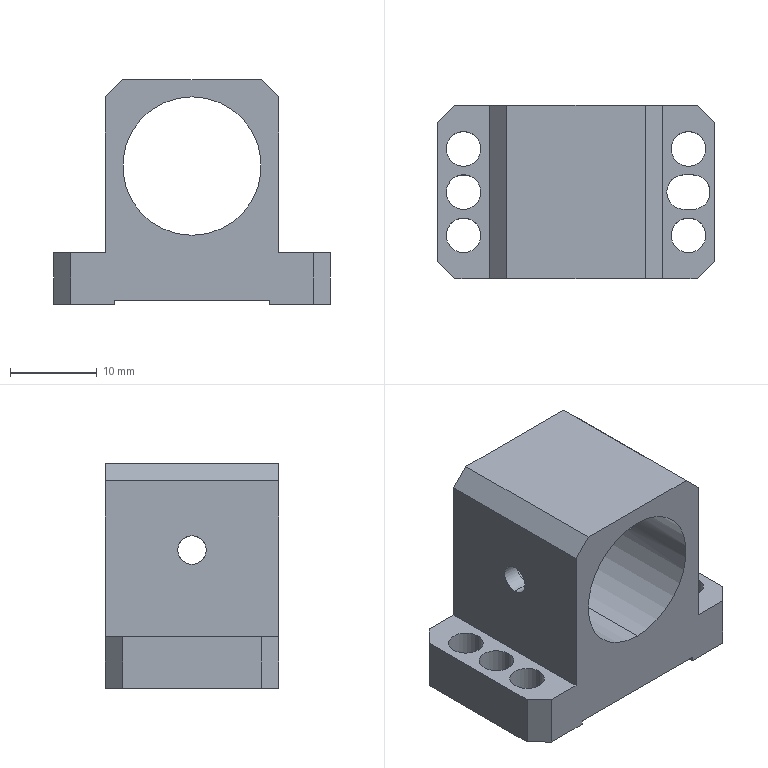NC program | NX | posted with a generic post | part box 32 x 20 x 26 mm
Lines 2153 to 2499 of 2499:
(PLANAR_MILL_COPY_COPY_1_COPY , TOOL : D6A45)
N4280 T07 M6
N4282 G54
N4284 G17 G0 G90 X12.87 Y6.2 B0. C0. S9500 M3
N4286 G43 Z30. H7
N4288 Z0.5
N4290 G94 G1 X12.73 Z0.462 F1250.
N4292 X12.13 Y5.87 Z0.279
N4294 X11.8 Y5.27 Z0.096
N4296 Y4.73 Z-0.049
N4298 X12.13 Y4.13 Z-0.233
N4300 X12.73 Y3.8 Z-0.416
N4302 X13.27 Z-0.561
N4304 X13.87 Y4.13 Z-0.744
N4306 X14.2 Y4.73 Z-0.928
N4308 Y5. Z-1.
N4310 G3 X13. Y6.2 R1.2
N4312 X14.2 Y5. R-1.2
N4314 X13.7 Y5.866 R1.
N4316 G1 Z0.5
N4318 G0 Z30.
N4320 X13.5 Y0.
N4322 Z0.5
N4324 G1 Z-1.
N4326 X13.866 Y0.7
N4328 G3 X13. Y1.2 R1.
N4330 G1 X12.5
N4332 G3 X11.3 Y0. R1.2
N4334 X12.5 Y-1.2 R1.2
N4336 G1 X13.5
N4338 G3 X14.7 Y0. R1.2
N4340 X13.5 Y1.2 R1.2
N4342 G1 X13.
N4344 G3 X12.134 Y0.7 R1.
N4346 G1 X12.5 Y0.
N4348 Z0.5
N4350 G0 Z30.
N4352 X12.87 Y-3.8
N4354 Z0.5
N4356 G1 X12.73 Z0.462
N4358 X12.13 Y-4.13 Z0.279
N4360 X11.8 Y-4.73 Z0.096
N4362 Y-5.27 Z-0.049
N4364 X12.13 Y-5.87 Z-0.233
N4366 X12.73 Y-6.2 Z-0.416
N4368 X13.27 Z-0.561
N4370 X13.87 Y-5.87 Z-0.744
N4372 X14.2 Y-5.27 Z-0.928
N4374 Y-5. Z-1.
N4376 G3 X13. Y-3.8 R1.2
N4378 X14.2 Y-5. R-1.2
N4380 X13.7 Y-4.134 R1.
N4382 G1 Z0.5
N4384 G0 Z30.
N4386 X9.263 Y12.184
N4388 Z0.5
N4390 G1 Z-1.
N4392 X9.207 Y11.72
N4394 G3 X9.6 Y10.8 R1.
N4396 G1 X13.917
N4398 G2 X14.624 Y10.507 R1.
N4400 G1 X16.507 Y8.624
N4402 G2 X16.8 Y7.917 R1.
N4404 G1 Y-7.917
N4406 G2 X16.507 Y-8.624 R1.
N4408 G1 X14.624 Y-10.507
N4410 G2 X13.917 Y-10.8 R1.
N4412 G1 X9.6
N4414 G3 X9.207 Y-11.72 R1.
N4416 G1 X9.263 Y-12.184
N4418 Z0.5
N4420 G0 Z30.
N4422 X-9.263
N4424 Z0.5
N4426 G1 Z-1.
N4428 X-9.207 Y-11.72
N4430 G3 X-9.6 Y-10.8 R1.
N4432 G1 X-13.917
N4434 G2 X-14.624 Y-10.507 R1.
N4436 G1 X-16.507 Y-8.624
N4438 G2 X-16.8 Y-7.917 R1.
N4440 G1 Y7.917
N4442 G2 X-16.507 Y8.624 R1.
N4444 G1 X-14.624 Y10.507
N4446 G2 X-13.917 Y10.8 R1.
N4448 G1 X-9.6
N4450 G3 X-9.207 Y11.72 R1.
N4452 G1 X-9.263 Y12.184
N4454 Z0.5
N4456 G0 Z30.
N4458 X-12.87 Y-6.2
N4460 Z0.5
N4462 G1 X-12.73 Z0.462
N4464 X-12.13 Y-5.87 Z0.279
N4466 X-11.8 Y-5.27 Z0.096
N4468 Y-4.73 Z-0.049
N4470 X-12.13 Y-4.13 Z-0.233
N4472 X-12.73 Y-3.8 Z-0.416
N4474 X-13.27 Z-0.561
N4476 X-13.87 Y-4.13 Z-0.744
N4478 X-14.2 Y-4.73 Z-0.928
N4480 Y-5. Z-1.
N4482 G3 X-13. Y-6.2 R1.2
N4484 X-14.2 Y-5. R-1.2
N4486 X-13.7 Y-5.866 R1.
N4488 G1 Z0.5
N4490 G0 Z30.
N4492 X-12.87 Y-1.2
N4494 Z0.5
N4496 G1 X-12.73 Z0.462
N4498 X-12.13 Y-0.87 Z0.279
N4500 X-11.8 Y-0.27 Z0.096
N4502 Y0.27 Z-0.049
N4504 X-12.13 Y0.87 Z-0.233
N4506 X-12.73 Y1.2 Z-0.416
N4508 X-13.27 Z-0.561
N4510 X-13.87 Y0.87 Z-0.744
N4512 X-14.2 Y0.27 Z-0.928
N4514 Y0. Z-1.
N4516 G3 X-13. Y-1.2 R1.2
N4518 X-14.2 Y0. R-1.2
N4520 X-13.7 Y-0.866 R1.
N4522 G1 Z0.5
N4524 G0 Z30.
N4526 X-12.87 Y3.8
N4528 Z0.5
N4530 G1 X-12.73 Z0.462
N4532 X-12.13 Y4.13 Z0.279
N4534 X-11.8 Y4.73 Z0.096
N4536 Y5.27 Z-0.049
N4538 X-12.13 Y5.87 Z-0.233
N4540 X-12.73 Y6.2 Z-0.416
N4542 X-13.27 Z-0.561
N4544 X-13.87 Y5.87 Z-0.744
N4546 X-14.2 Y5.27 Z-0.928
N4548 Y5. Z-1.
N4550 G3 X-13. Y3.8 R1.2
N4552 X-14.2 Y5. R-1.2
N4554 X-13.7 Y4.134 R1.
N4556 G1 Z0.5
N4558 G0 Z30.
(PLANAR_MILL_COPY_COPY_1_COPY_COPY , TOOL : D6A45)
N4560 X6.721 Y-12.246
N4562 Z0.
N4564 G1 Z-1.5
N4566 X7.055 Y-11.794
N4568 G3 X7.167 Y-10.8 R1.
N4570 G1 X-7.167
N4572 G3 X-7.055 Y-11.794 R1.
N4574 G1 X-6.721 Y-12.246
N4576 Z0.
N4578 G0 Z30.
N4580 Y12.246
N4582 Z0.
N4584 G1 Z-1.5
N4586 X-7.055 Y11.794
N4588 G3 X-7.167 Y10.8 R1.
N4590 G1 X7.167
N4592 G3 X7.055 Y11.794 R1.
N4594 G1 X6.721 Y12.246
N4596 Z0.
N4598 G0 Z30.
N4600 M5
(刀补3 , TOOL : D3)
N4602 T03 M6
N4604 G54
N4606 G17 G0 G90 X-12.942 Y-0.138 B0. C0. S9500 M3
N4608 G43 Z30. H3
N4610 Z-1.
N4612 G94 G1 Z-2. F1000.
N4614 G41 X-12.713 Y-0.346 D3
N4616 X-12.628 Y-0.253 F1200.
N4618 G3 X-12.783 Y0.394 R0.45
N4620 G1 X-12.812 Y0.399
N4622 X-12.829 Y0.416
N4624 G3 X-13.372 Y-0.253 R0.45
N4626 G1 X-13.288 Y-0.346
N4628 G3 X-12.713 Y-0.346 R0.45
N4630 G1 X-12.645 Y-0.265 Z-2.099
N4632 X-12.618 Y-0.221 Z-2.149
N4634 X-12.578 Y-0.156 Z-2.222
N4636 X-12.564 Y-0.079 Z-2.297
N4638 X-12.557 Y-0.002 Z-2.371
N4640 X-12.564 Y0.075 Z-2.444
N4642 X-12.589 Y0.163 Z-2.531
N4644 X-12.608 Y0.204 Z-2.575
N4646 X-12.623 Y0.231 Z-2.605
N4648 X-12.661 Y0.282 Z-2.667
N4650 X-12.731 Y0.352 Z-2.761
N4652 X-12.771 Y0.378 Z-2.808
N4654 X-12.795 Y0.391 Z-2.835
N4656 X-12.845 Y0.414 Z-2.889
N4658 X-12.936 Y0.437 Z-2.978
N4660 X-13.012 Y0.443 Z-3.052
N4662 X-13.073 Y0.436 Z-3.111
N4664 X-13.164 Y0.412 Z-3.2
N4666 X-13.231 Y0.377 Z-3.274
N4668 X-13.28 Y0.34 Z-3.333
N4670 X-13.351 Y0.269 Z-3.427
N4672 X-13.378 Y0.229 Z-3.475
N4674 X-13.392 Y0.205 Z-3.502
N4676 X-13.414 Y0.155 Z-3.556
N4678 X-13.438 Y0.063 Z-3.645
N4680 X-13.443 Y0.017 Z-3.689
N4682 X-13.442 Y-0.013 Z-3.719
N4684 X-13.436 Y-0.073 Z-3.778
N4686 X-13.422 Y-0.13 Z-3.833
N4688 X-13.402 Y-0.184 Z-3.889
N4690 X-13.376 Y-0.235 Z-3.944
N4692 X-13.344 Y-0.284 Z-4.
N4694 X-13.288 Y-0.346
N4696 G3 X-12.713 Y-0.346 R0.45
N4698 G1 X-12.646 Y-0.265 Z-4.099
N4700 X-12.618 Y-0.221 Z-4.149
N4702 X-12.578 Y-0.156 Z-4.222
N4704 X-12.564 Y-0.079 Z-4.297
N4706 X-12.557 Y-0.002 Z-4.371
N4708 X-12.564 Y0.075 Z-4.444
N4710 X-12.589 Y0.163 Z-4.531
N4712 X-12.608 Y0.204 Z-4.575
N4714 X-12.623 Y0.231 Z-4.605
N4716 X-12.661 Y0.282 Z-4.667
N4718 X-12.731 Y0.352 Z-4.761
N4720 X-12.771 Y0.378 Z-4.808
N4722 X-12.795 Y0.391 Z-4.835
N4724 X-12.845 Y0.414 Z-4.889
N4726 X-12.936 Y0.437 Z-4.978
N4728 X-13.012 Y0.443 Z-5.052
N4730 X-13.073 Y0.436 Z-5.111
N4732 X-13.164 Y0.412 Z-5.2
N4734 X-13.231 Y0.377 Z-5.274
N4736 X-13.28 Y0.34 Z-5.333
N4738 X-13.351 Y0.269 Z-5.427
N4740 X-13.378 Y0.229 Z-5.475
N4742 X-13.392 Y0.205 Z-5.502
N4744 X-13.414 Y0.155 Z-5.556
N4746 X-13.438 Y0.063 Z-5.645
N4748 X-13.442 Y0.018 Z-5.689
N4750 Y-0.013 Z-5.719
N4752 X-13.436 Y-0.073 Z-5.778
N4754 X-13.422 Y-0.13 Z-5.833
N4756 X-13.402 Y-0.184 Z-5.889
N4758 X-13.376 Y-0.235 Z-5.944
N4760 X-13.344 Y-0.284 Z-6.
N4762 X-13.288 Y-0.346
N4764 G3 X-12.713 Y-0.346 R0.45
N4766 G1 X-12.628 Y-0.253
N4768 G3 X-12.783 Y0.394 R0.45
N4770 G1 X-12.812 Y0.399
N4772 X-12.829 Y0.416
N4774 G3 X-13.372 Y-0.253 R0.45
N4776 G1 X-13.344 Y-0.284
N4778 G40
N4780 X-13.122 Y-0.082
N4782 Z-5.
N4784 G0 Z30.
N4786 X12.5 Y-0.15
N4788 Z-1.
N4790 G1 Z-2. F1000.
N4792 G41 Y-0.45
N4794 X13.5 F1200.
N4796 G3 X13.95 Y0. R0.45
N4798 X13.5 Y0.45 R0.45
N4800 G1 X12.5
N4802 G3 X12.05 Y0. R0.45
N4804 X12.5 Y-0.45 R0.45
N4806 G1 X13.345 Z-2.467
N4808 X13.465 Y-0.446 Z-2.533
N4810 X13.584 Y-0.436 Z-2.598
N4812 X13.659 Y-0.414 Z-2.643
N4814 X13.696 Y-0.396 Z-2.667
N4816 X13.782 Y-0.339 Z-2.724
N4818 X13.819 Y-0.306 Z-2.752
N4820 X13.837 Y-0.285 Z-2.768
N4822 X13.871 Y-0.24 Z-2.8
N4824 X13.916 Y-0.154 Z-2.854
N4826 X13.928 Y-0.108 Z-2.881
N4828 X13.935 Y-0.078 Z-2.898
N4830 X13.942 Y-0.017 Z-2.933
N4832 X13.936 Y0.077 Z-2.986
N4834 X13.925 Y0.122 Z-3.012
N4836 X13.915 Y0.152 Z-3.03
N4838 X13.887 Y0.21 Z-3.067
N4840 X13.83 Y0.294 Z-3.122
N4842 X13.796 Y0.329 Z-3.15
N4844 X13.773 Y0.346 Z-3.167
N4846 X13.726 Y0.38 Z-3.2
N4848 X13.667 Y0.411 Z-3.238
N4850 X13.592 Y0.434 Z-3.282
N4852 X13.5 Y0.444 Z-3.333
N4854 X13.379 Y0.45 Z-3.4
N4856 X12.655 Z-3.8
N4858 X12.535 Y0.446 Z-3.867
N4860 X12.474 Y0.442 Z-3.9
N4862 X12.415 Y0.436 Z-3.933
N4864 X12.358 Y0.418 Z-3.967
N4866 X12.3 Y0.403 Z-4.
N4868 G3 X12.5 Y-0.45 R0.45
N4870 G1 X13.345 Z-4.467
N4872 X13.465 Y-0.446 Z-4.533
N4874 X13.584 Y-0.436 Z-4.598
N4876 X13.659 Y-0.414 Z-4.643
N4878 X13.696 Y-0.396 Z-4.667
N4880 X13.782 Y-0.34 Z-4.724
N4882 X13.819 Y-0.306 Z-4.752
N4884 X13.837 Y-0.285 Z-4.768
N4886 X13.871 Y-0.24 Z-4.8
N4888 X13.915 Y-0.154 Z-4.854
N4890 X13.928 Y-0.108 Z-4.881
N4892 X13.935 Y-0.078 Z-4.898
N4894 X13.942 Y-0.017 Z-4.933
N4896 X13.936 Y0.077 Z-4.986
N4898 X13.925 Y0.122 Z-5.012
N4900 X13.915 Y0.152 Z-5.03
N4902 X13.887 Y0.21 Z-5.067
N4904 X13.83 Y0.294 Z-5.122
N4906 X13.796 Y0.328 Z-5.15
N4908 X13.773 Y0.346 Z-5.167
N4910 X13.726 Y0.38 Z-5.2
N4912 X13.667 Y0.411 Z-5.238
N4914 X13.592 Y0.434 Z-5.282
N4916 X13.5 Y0.444 Z-5.333
N4918 X13.379 Y0.45 Z-5.4
N4920 X12.655 Z-5.8
N4922 X12.535 Y0.446 Z-5.867
N4924 X12.474 Y0.442 Z-5.9
N4926 X12.415 Y0.436 Z-5.933
N4928 X12.358 Y0.418 Z-5.967
N4930 X12.3 Y0.403 Z-6.
N4932 G3 X12.5 Y-0.45 R0.45
N4934 G1 X13.5
N4936 G3 X13.95 Y0. R0.45
N4938 X13.5 Y0.45 R0.45
N4940 G1 X12.5
N4942 G3 X12.3 Y0.403 R0.45
N4944 G40
N4946 G1 X12.433 Y0.134
N4948 Z-5.
N4950 G0 Z30.
N4952 M5
N4954 M2